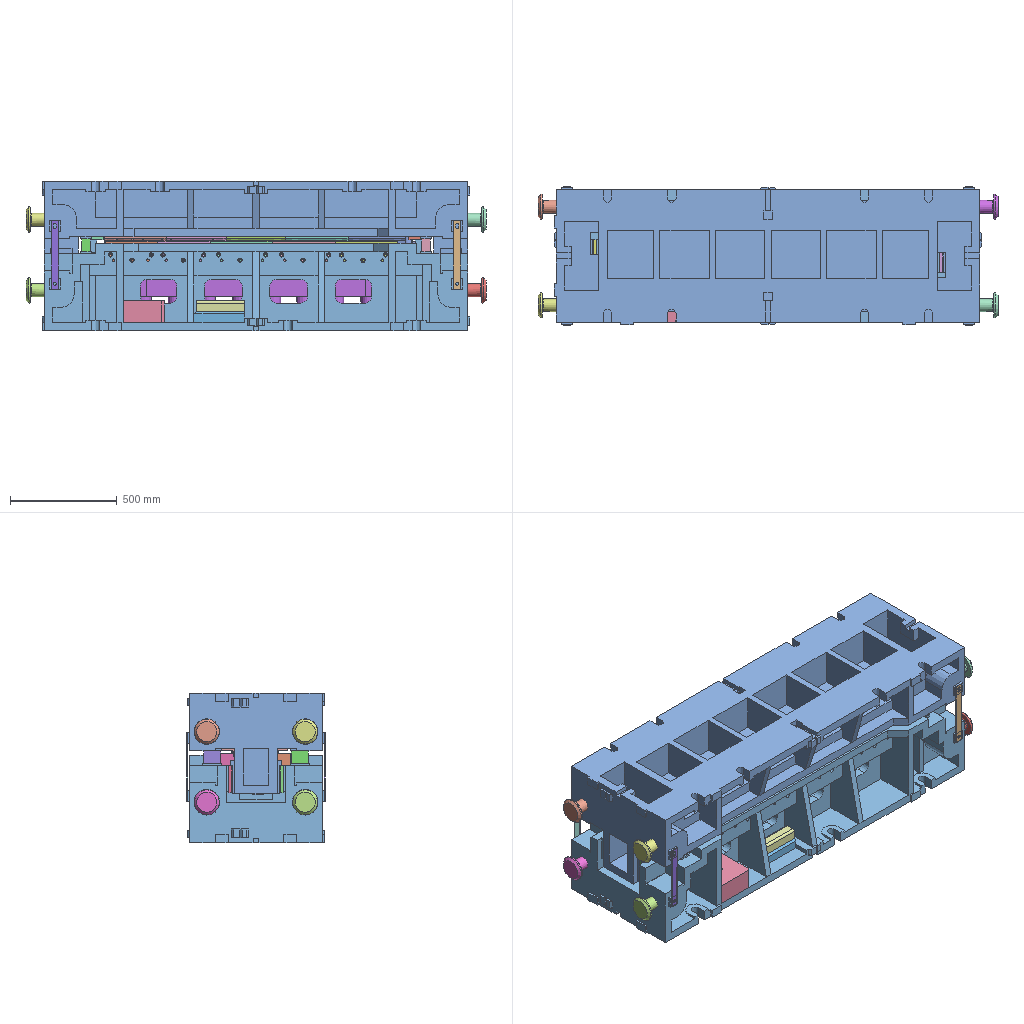Assembly | NX | 100 different items | 100 placed | box 2150 x 646 x 700 mm
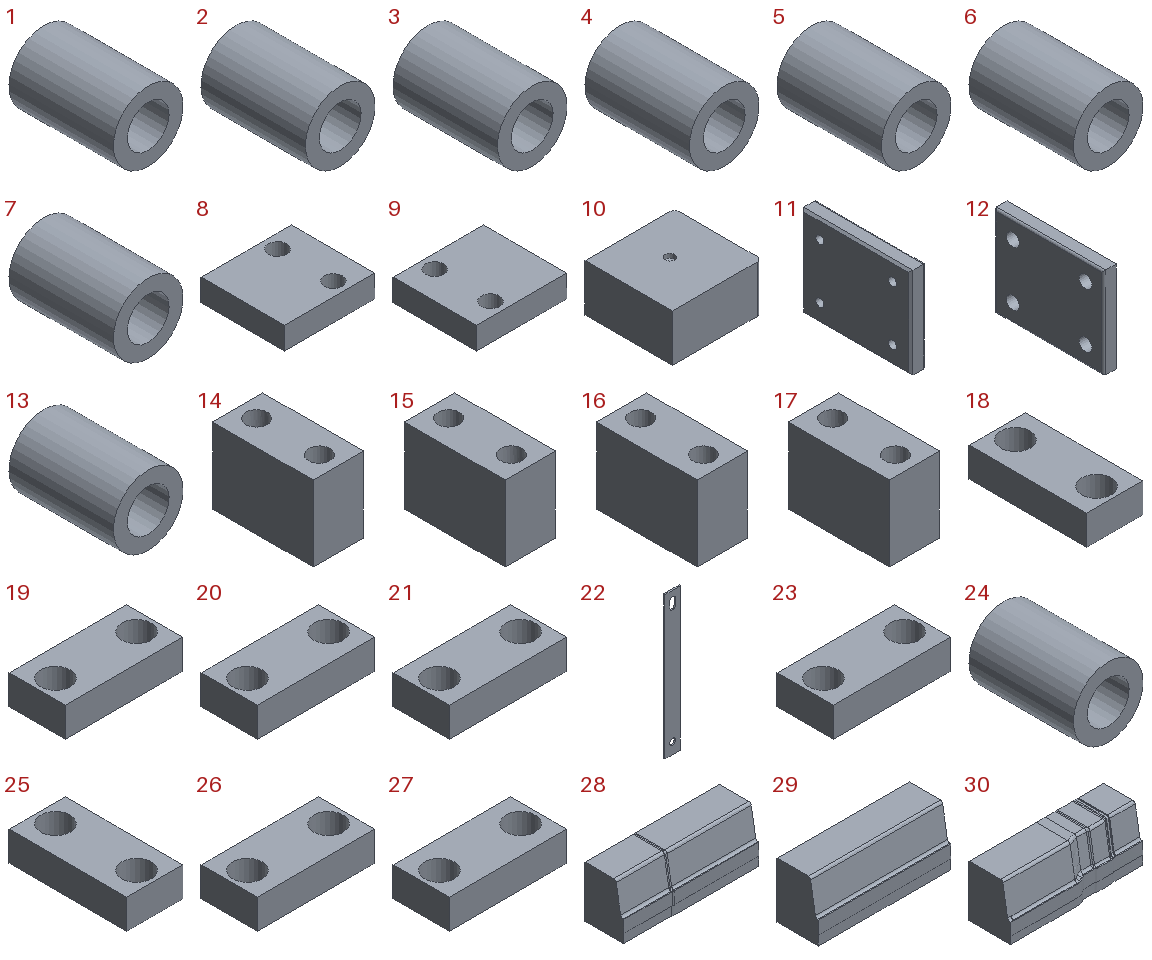Parts list (item | quantity | size | volume | features):
1 | x1 | 20 x 30 x 20 mm | 6032 mm3 | features solid 2
2 | x1 | 20 x 30 x 20 mm | 6032 mm3 | features solid 2
3 | x1 | 20 x 30 x 20 mm | 6032 mm3 | features solid 2
4 | x1 | 20 x 30 x 20 mm | 6032 mm3 | features solid 2
5 | x1 | 20 x 30 x 20 mm | 6032 mm3 | features solid 2
6 | x1 | 20 x 30 x 20 mm | 6032 mm3 | features solid 2
7 | x1 | 20 x 30 x 20 mm | 6032 mm3 | features solid 2
8 | x1 | 65 x 60 x 16 mm | 58153 mm3 | features solid 2
9 | x1 | 65 x 60 x 16 mm | 58153 mm3 | features solid 2
10 | x1 | 190 x 185 x 100 mm | 3507251 mm3 | features solid 2
11 | x1 | 20 x 150 x 125 mm | 356923 mm3 | features solid 2
12 | x1 | 20 x 150 x 125 mm | 356923 mm3 | features solid 2
13 | x1 | 20 x 30 x 20 mm | 6032 mm3 | features solid 2
14 | x1 | 40 x 80 x 60 mm | 176638 mm3 | features solid 2
15 | x1 | 40 x 80 x 60 mm | 176638 mm3 | features solid 2
16 | x1 | 40 x 80 x 60 mm | 176638 mm3 | features solid 2
17 | x1 | 40 x 80 x 60 mm | 176638 mm3 | features solid 2
18 | x1 | 38 x 80 x 20 mm | 50411 mm3 | features solid 2
19 | x1 | 80 x 38 x 20 mm | 50411 mm3 | features solid 2
20 | x1 | 80 x 38 x 20 mm | 50411 mm3 | features solid 2
21 | x1 | 80 x 38 x 20 mm | 50411 mm3 | features solid 2
22 | x1 | 35 x 3 x 320 mm | 32235 mm3 | features solid 2
23 | x1 | 80 x 38 x 20 mm | 50411 mm3 | features solid 2
24 | x1 | 20 x 30 x 20 mm | 6032 mm3 | features solid 2
25 | x1 | 38 x 80 x 20 mm | 50411 mm3 | features solid 2
26 | x1 | 80 x 38 x 20 mm | 50411 mm3 | features solid 2
27 | x1 | 80 x 38 x 20 mm | 50411 mm3 | features solid 2
28 | x1 | 280 x 82.143 x 107.133 mm | 2215544 mm3 | features solid 2
29 | x1 | 255 x 81.128 x 107.133 mm | 1996721 mm3 | features solid 2
30 | x1 | 280 x 87.161 x 107.138 mm | 2279112 mm3 | features solid 2
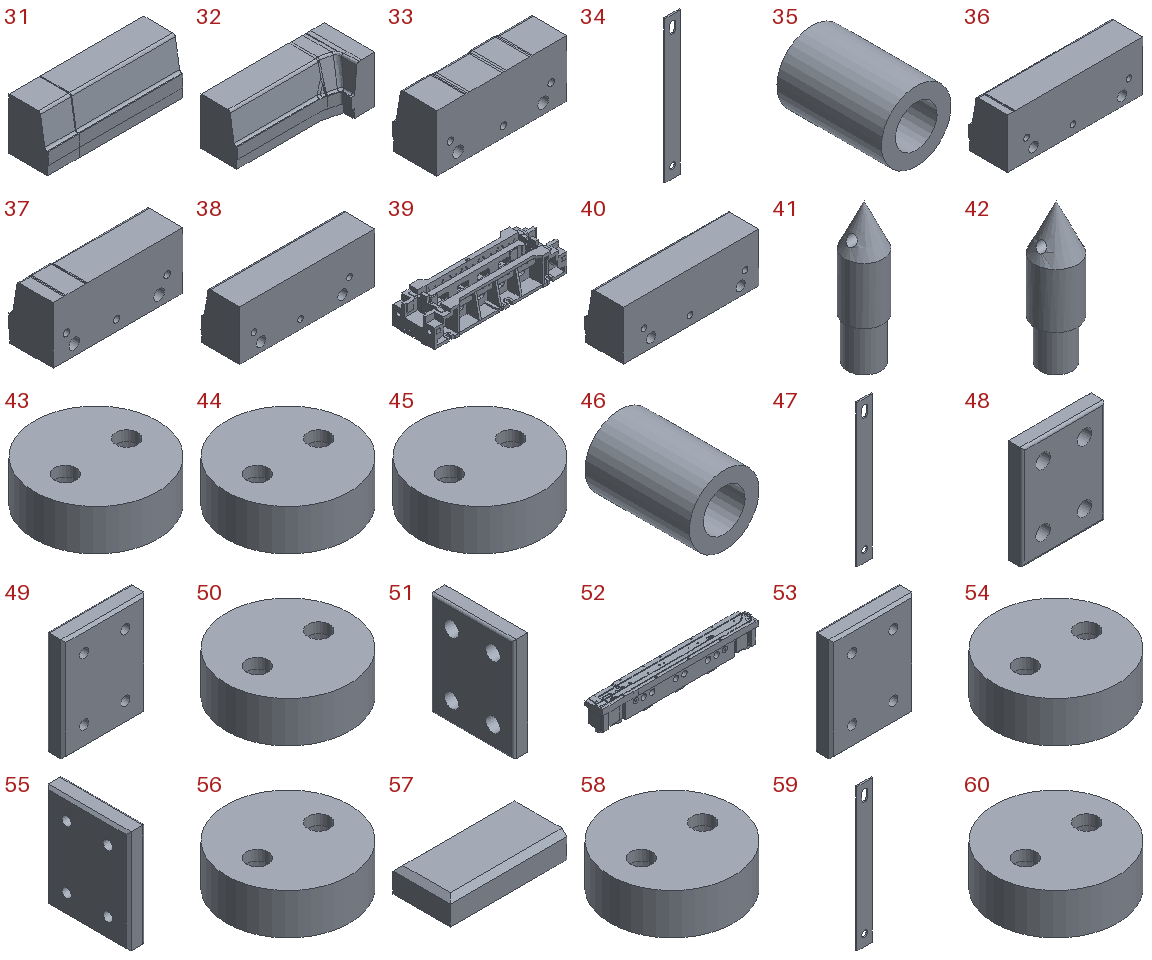31 | x1 | 280 x 81.346 x 107.138 mm | 2196752 mm3 | features solid 2
32 | x1 | 280 x 115 x 107.135 mm | 2442427 mm3 | features solid 2
33 | x1 | 245 x 84.549 x 107.259 mm | 1984457 mm3 | features solid 2
34 | x1 | 35 x 3 x 320 mm | 32235 mm3 | features solid 2
35 | x1 | 20 x 30 x 20 mm | 6032 mm3 | features solid 2
36 | x1 | 290 x 83.721 x 107.133 mm | 2375336 mm3 | features solid 2
37 | x1 | 245 x 83.473 x 107.229 mm | 1994920 mm3 | features solid 2
38 | x1 | 290 x 83.705 x 107.133 mm | 2376926 mm3 | features solid 2
39 | x1 | 2000 x 640 x 425 mm | 163396504 mm3 | features solid 2
40 | x1 | 295 x 83.706 x 107.133 mm | 2418413 mm3 | features solid 2
41 | x1 | 13.7 x 13.7 x 50 mm | 5325 mm3 | features solid 2
42 | x1 | 15.7 x 15.7 x 52 mm | 6599 mm3 | features solid 2
43 | x1 | 60 x 60 x 20 mm | 48467 mm3 | features solid 2
44 | x1 | 60 x 60 x 20 mm | 48467 mm3 | features solid 2
45 | x1 | 60 x 60 x 20 mm | 48467 mm3 | features solid 2
46 | x1 | 20 x 30 x 20 mm | 6032 mm3 | features solid 2
47 | x1 | 35 x 3 x 320 mm | 32235 mm3 | features solid 2
48 | x1 | 100 x 20 x 125 mm | 232566 mm3 | features solid 2
49 | x1 | 100 x 20 x 125 mm | 232566 mm3 | features solid 2
50 | x1 | 60 x 60 x 20 mm | 48467 mm3 | features solid 2
51 | x1 | 20 x 100 x 125 mm | 232566 mm3 | features solid 2
52 | x1 | 1460 x 171.859 x 235.617 mm | 41885749 mm3 | features solid 2
53 | x1 | 100 x 20 x 125 mm | 232566 mm3 | features solid 2
54 | x1 | 60 x 60 x 20 mm | 48467 mm3 | features solid 2
55 | x1 | 20 x 100 x 125 mm | 232566 mm3 | features solid 2
56 | x1 | 60 x 60 x 20 mm | 48467 mm3 | features solid 2
57 | x1 | 235 x 115 x 50 mm | 1322667 mm3 | features solid 2
58 | x1 | 60 x 60 x 20 mm | 48467 mm3 | features solid 2
59 | x1 | 35 x 3 x 320 mm | 32235 mm3 | features solid 2
60 | x1 | 60 x 60 x 20 mm | 48467 mm3 | features solid 2
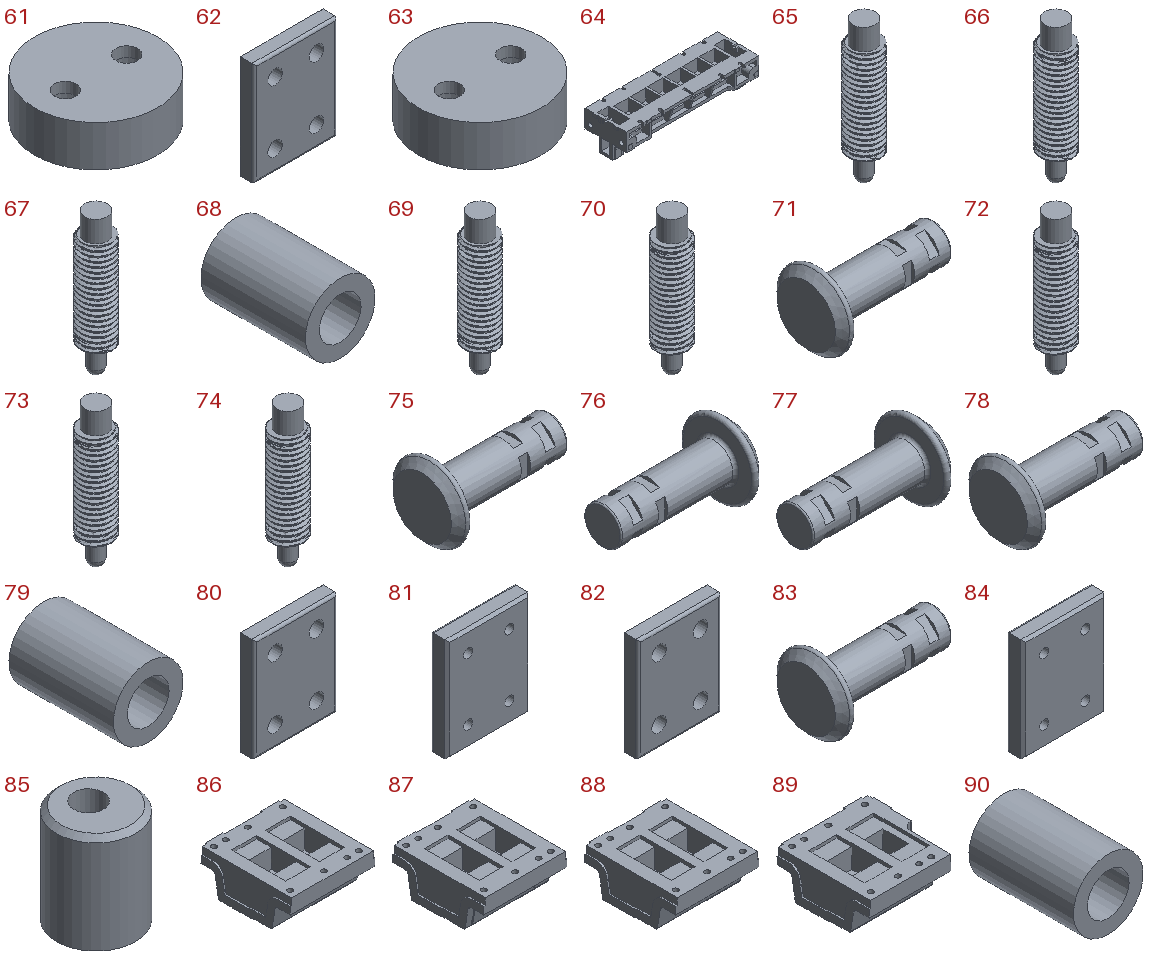61 | x1 | 60 x 60 x 20 mm | 48467 mm3 | features solid 2
62 | x1 | 100 x 20 x 125 mm | 232566 mm3 | features solid 2
63 | x1 | 60 x 60 x 20 mm | 48467 mm3 | features solid 2
64 | x1 | 2000 x 640 x 475 mm | 146467854 mm3 | features solid 2
65 | x1 | 11.998 x 11.997 x 53 mm | 4026 mm3 | features solid 2
66 | x1 | 11.998 x 11.997 x 53 mm | 4026 mm3 | features solid 2
67 | x1 | 11.998 x 11.997 x 53 mm | 4026 mm3 | features solid 2
68 | x1 | 20 x 30 x 20 mm | 6032 mm3 | features solid 2
69 | x1 | 11.998 x 11.997 x 53 mm | 4026 mm3 | features solid 2
70 | x1 | 11.998 x 11.997 x 53 mm | 4026 mm3 | features solid 2
71 | x1 | 205 x 120 x 120 mm | 705223 mm3 | features solid 2
72 | x1 | 11.998 x 11.997 x 53 mm | 4026 mm3 | features solid 2
73 | x1 | 11.998 x 11.997 x 53 mm | 4026 mm3 | features solid 2
74 | x1 | 11.998 x 11.997 x 53 mm | 4026 mm3 | features solid 2
75 | x1 | 205 x 120 x 120 mm | 705223 mm3 | features solid 2
76 | x1 | 205 x 120 x 120 mm | 705223 mm3 | features solid 2
77 | x1 | 205 x 120 x 120 mm | 705223 mm3 | features solid 2
78 | x1 | 205 x 120 x 120 mm | 705223 mm3 | features solid 2
79 | x1 | 20 x 30 x 20 mm | 6032 mm3 | features solid 2
80 | x1 | 100 x 20 x 125 mm | 232566 mm3 | features solid 2
81 | x1 | 100 x 20 x 125 mm | 232566 mm3 | features solid 2
82 | x1 | 100 x 20 x 125 mm | 232566 mm3 | features solid 2
83 | x1 | 205 x 120 x 120 mm | 705223 mm3 | features solid 2
84 | x1 | 100 x 20 x 125 mm | 232566 mm3 | features solid 2
85 | x1 | 16 x 16 x 20.5 mm | 3091 mm3 | features solid 2
86 | x1 | 290 x 310 x 126.004 mm | 7008065 mm3 | features solid 2
87 | x1 | 280 x 310 x 126.004 mm | 6791703 mm3 | features solid 2
88 | x1 | 280.327 x 310 x 126.004 mm | 6807887 mm3 | features solid 2
89 | x1 | 305 x 310 x 125.996 mm | 6829711 mm3 | features solid 2
90 | x1 | 20 x 30 x 20 mm | 6032 mm3 | features solid 2
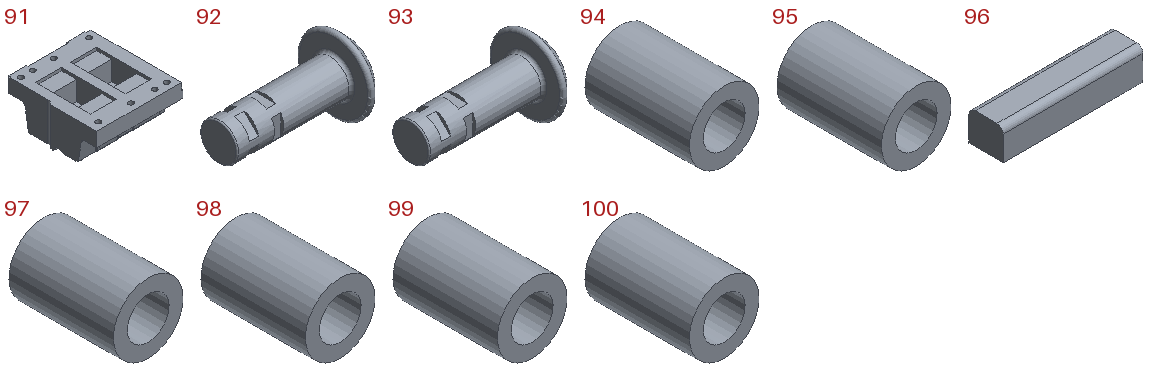91 | x1 | 290 x 310 x 129.453 mm | 6904200 mm3 | features solid 2
92 | x1 | 205 x 120 x 120 mm | 705223 mm3 | features solid 2
93 | x1 | 205 x 120 x 120 mm | 705223 mm3 | features solid 2
94 | x1 | 20 x 30 x 20 mm | 6032 mm3 | features solid 2
95 | x1 | 20 x 30 x 20 mm | 6032 mm3 | features solid 2
96 | x1 | 225 x 55 x 50 mm | 609093 mm3 | features solid 2
97 | x1 | 20 x 30 x 20 mm | 6032 mm3 | features solid 2
98 | x1 | 20 x 30 x 20 mm | 6032 mm3 | features solid 2
99 | x1 | 20 x 30 x 20 mm | 6032 mm3 | features solid 2
100 | x1 | 20 x 30 x 20 mm | 6032 mm3 | features solid 2